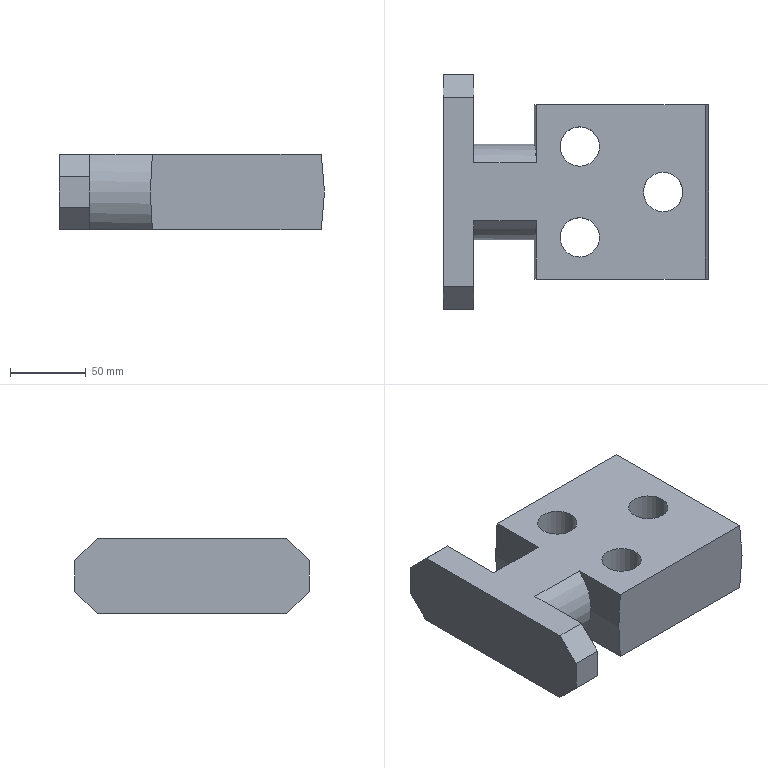Part | NX | features CHPL63_1 2 | 1 solid | 97 faces | box 175 x 155 x 50 mm | volume 830301 mm3 | plane 69 | cylinder 28 | commonest cylinder face diameters 26 x3 10.09 x2 63 x2 5.912 x1 5.927 x1 6.108 x1